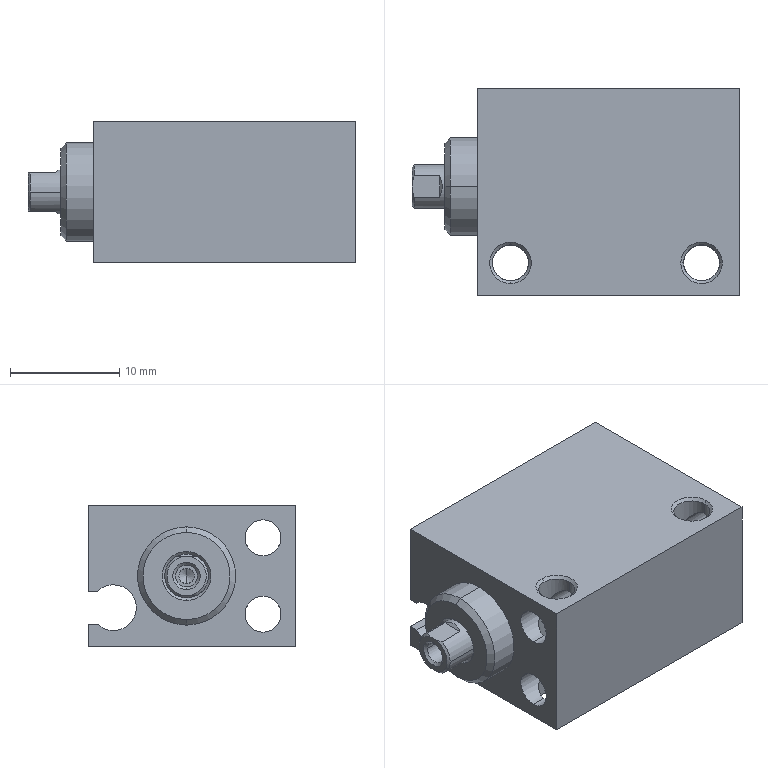Part | STEP file | Compact free-mount cylinder MU6x6S | 2 solids | 103 faces | box 30 x 19 x 13 mm | volume 4914 mm3 | cylinder 53 | plane 26 | cone 24 | commonest cylinder face diameters 3.3 x24 1 x4 2.459 x4 4 x4 6 x4 4.2 x3